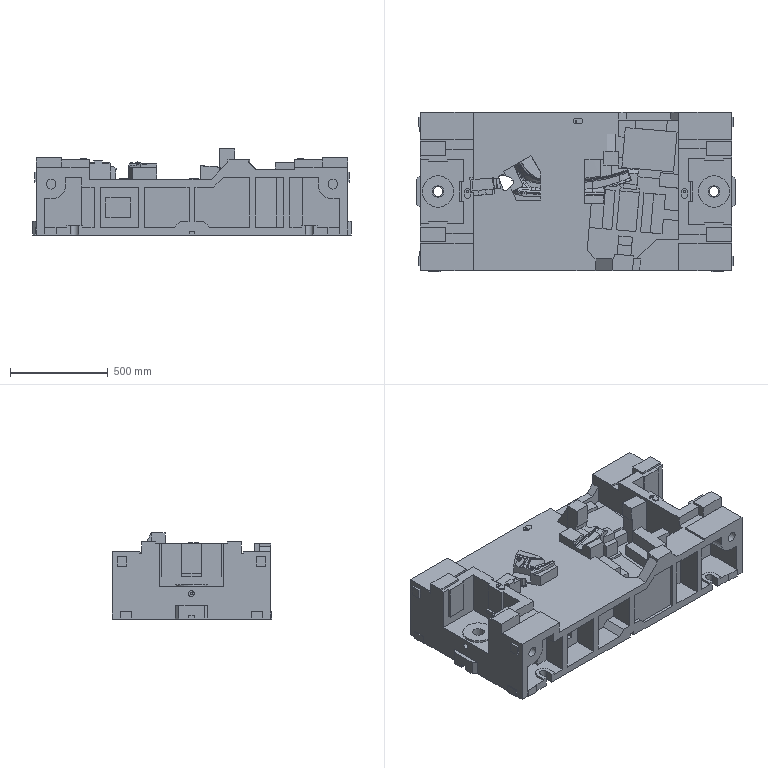Part | NX | features solid 2 | 1 solid | 690 faces | box 1630 x 815 x 440 mm | volume 191809441 mm3 | plane 524 | spline 125 | cylinder 41 | commonest cylinder face diameters 30 x9 50 x6 10 x5 40 x5 80 x4 140 x4